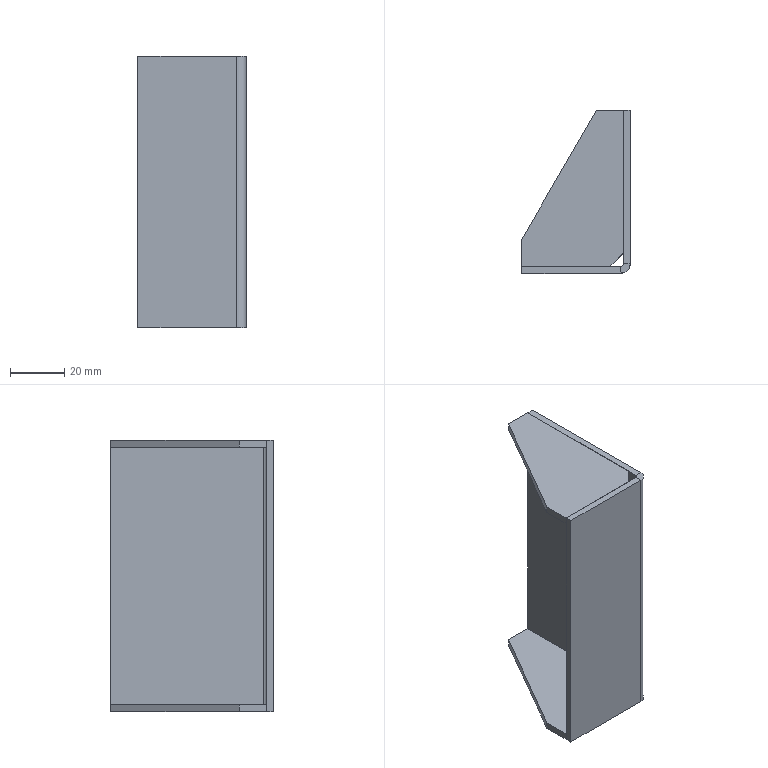Part | SolidWorks | features BaseBody 3 | 3 solids | 30 faces | box 40 x 60 x 100 mm | volume 31587 mm3 | plane 28 | cylinder 2 | commonest cylinder face diameters 2 x1 7 x1
STEP:
#1=CARTESIAN_POINT('',(-3.5,-57.5,-50.));
#2=VERTEX_POINT('',#1);
#3=CARTESIAN_POINT('',(-40.,-57.5,-50.));
#4=VERTEX_POINT('',#3);
#5=CARTESIAN_POINT('',(0.,-57.5,-50.));
#6=DIRECTION('',(-1.,0.,0.));
#7=VECTOR('',#6,1000.);
#8=LINE('',#5,#7);
#9=EDGE_CURVE('',#2,#4,#8,.T.);
#10=ORIENTED_EDGE('',*,*,#9,.F.);
#11=CARTESIAN_POINT('',(-3.5,-60.,-50.));
#12=VERTEX_POINT('',#11);
#13=CARTESIAN_POINT('',(-3.5,-57.5,-50.));
#14=DIRECTION('',(0.,-1.,0.));
#15=VECTOR('',#14,1000.);
#16=LINE('',#13,#15);
#17=EDGE_CURVE('',#2,#12,#16,.T.);
#18=ORIENTED_EDGE('',*,*,#17,.T.);
#19=CARTESIAN_POINT('',(-40.,-60.,-50.));
#20=VERTEX_POINT('',#19);
#21=CARTESIAN_POINT('',(0.,-60.,-50.));
#22=DIRECTION('',(-1.,0.,0.));
#23=VECTOR('',#22,1000.);
#24=LINE('',#21,#23);
#25=EDGE_CURVE('',#12,#20,#24,.T.);
#26=ORIENTED_EDGE('',*,*,#25,.T.);
#27=CARTESIAN_POINT('',(-40.,-60.,-50.));
#28=DIRECTION('',(0.,1.,0.));
#29=VECTOR('',#28,1000.);
#30=LINE('',#27,#29);
#31=EDGE_CURVE('',#20,#4,#30,.T.);
#32=ORIENTED_EDGE('',*,*,#31,.T.);
#33=EDGE_LOOP('',(#10,#18,#26,#32));
#34=FACE_OUTER_BOUND('',#33,.T.);
#35=CARTESIAN_POINT('',(-3.5,-56.5,-50.));
#36=DIRECTION('',(0.,0.,1.));
#37=DIRECTION('',(1.,0.,0.));
#38=AXIS2_PLACEMENT_3D('',#35,#36,#37);
#39=PLANE('',#38);
#40=ADVANCED_FACE('',(#34),#39,.F.);
#41=CARTESIAN_POINT('',(-2.5,0.,50.));
#42=VERTEX_POINT('',#41);
#43=CARTESIAN_POINT('',(-2.5,-56.5,50.));
#44=VERTEX_POINT('',#43);
#45=CARTESIAN_POINT('',(-2.5,0.,50.));
#46=DIRECTION('',(0.,-1.,0.));
#47=VECTOR('',#46,1000.);
#48=LINE('',#45,#47);
#49=EDGE_CURVE('',#42,#44,#48,.T.);
#50=ORIENTED_EDGE('',*,*,#49,.T.);
#51=CARTESIAN_POINT('',(0.,-56.5,50.));
#52=VERTEX_POINT('',#51);
#53=CARTESIAN_POINT('',(-2.5,-56.5,50.));
#54=DIRECTION('',(1.,0.,0.));
#55=VECTOR('',#54,1000.);
#56=LINE('',#53,#55);
#57=EDGE_CURVE('',#44,#52,#56,.T.);
#58=ORIENTED_EDGE('',*,*,#57,.T.);
#59=CARTESIAN_POINT('',(0.,0.,50.));
#60=VERTEX_POINT('',#59);
#61=CARTESIAN_POINT('',(0.,0.,50.));
#62=DIRECTION('',(0.,-1.,0.));
#63=VECTOR('',#62,1000.);
#64=LINE('',#61,#63);
#65=EDGE_CURVE('',#60,#52,#64,.T.);
#66=ORIENTED_EDGE('',*,*,#65,.F.);
#67=CARTESIAN_POINT('',(-2.5,0.,50.));
#68=DIRECTION('',(1.,0.,0.));
#69=VECTOR('',#68,1000.);
#70=LINE('',#67,#69);
#71=EDGE_CURVE('',#42,#60,#70,.T.);
#72=ORIENTED_EDGE('',*,*,#71,.F.);
#73=EDGE_LOOP('',(#50,#58,#66,#72));
#74=FACE_OUTER_BOUND('',#73,.T.);
#75=CARTESIAN_POINT('',(-3.5,-56.5,50.));
#76=DIRECTION('',(0.,0.,1.));
#77=DIRECTION('',(1.,0.,0.));
#78=AXIS2_PLACEMENT_3D('',#75,#76,#77);
#79=PLANE('',#78);
#80=ADVANCED_FACE('',(#74),#79,.T.);
#81=CARTESIAN_POINT('',(-2.5,-56.5,-50.));
#82=VERTEX_POINT('',#81);
#83=CARTESIAN_POINT('',(-3.5,-56.5,-50.));
#84=DIRECTION('',(0.,0.,-1.));
#85=DIRECTION('',(1.,0.,0.));
#86=AXIS2_PLACEMENT_3D('',#83,#84,#85);
#87=CIRCLE('',#86,1.);
#88=EDGE_CURVE('',#82,#2,#87,.T.);
#89=ORIENTED_EDGE('',*,*,#88,.T.);
#90=CARTESIAN_POINT('',(-3.5,-57.5,50.));
#91=VERTEX_POINT('',#90);
#92=CARTESIAN_POINT('',(-3.5,-57.5,50.));
#93=DIRECTION('',(0.,0.,-1.));
#94=VECTOR('',#93,1000.);
#95=LINE('',#92,#94);
#96=EDGE_CURVE('',#91,#2,#95,.T.);
#97=ORIENTED_EDGE('',*,*,#96,.F.);
#98=CARTESIAN_POINT('',(-3.5,-56.5,50.));
#99=DIRECTION('',(0.,0.,-1.));
#100=DIRECTION('',(1.,0.,0.));
#101=AXIS2_PLACEMENT_3D('',#98,#99,#100);
#102=CIRCLE('',#101,1.);
#103=EDGE_CURVE('',#44,#91,#102,.T.);
#104=ORIENTED_EDGE('',*,*,#103,.F.);
#105=CARTESIAN_POINT('',(-2.5,-56.5,50.));
#106=DIRECTION('',(0.,0.,-1.));
#107=VECTOR('',#106,1000.);
#108=LINE('',#105,#107);
#109=EDGE_CURVE('',#44,#82,#108,.T.);
#110=ORIENTED_EDGE('',*,*,#109,.T.);
#111=EDGE_LOOP('',(#89,#97,#104,#110));
#112=FACE_OUTER_BOUND('',#111,.T.);
#113=CARTESIAN_POINT('',(-3.5,-56.5,50.));
#114=DIRECTION('',(0.,0.,-1.));
#115=DIRECTION('',(-1.,0.,0.));
#116=AXIS2_PLACEMENT_3D('',#113,#114,#115);
#117=CYLINDRICAL_SURFACE('',#116,1.);
#118=ADVANCED_FACE('',(#112),#117,.F.);
#119=CARTESIAN_POINT('',(-2.5,0.,-50.));
#120=VERTEX_POINT('',#119);
#121=CARTESIAN_POINT('',(-2.5,0.,-50.));
#122=DIRECTION('',(0.,-1.,0.));
#123=VECTOR('',#122,1000.);
#124=LINE('',#121,#123);
#125=EDGE_CURVE('',#120,#82,#124,.T.);
#126=ORIENTED_EDGE('',*,*,#125,.T.);
#127=ORIENTED_EDGE('',*,*,#109,.F.);
#128=ORIENTED_EDGE('',*,*,#49,.F.);
#129=CARTESIAN_POINT('',(-2.5,0.,50.));
#130=DIRECTION('',(0.,0.,-1.));
#131=VECTOR('',#130,1000.);
#132=LINE('',#129,#131);
#133=EDGE_CURVE('',#42,#120,#132,.T.);
#134=ORIENTED_EDGE('',*,*,#133,.T.);
#135=EDGE_LOOP('',(#126,#127,#128,#134));
#136=FACE_OUTER_BOUND('',#135,.T.);
#137=CARTESIAN_POINT('',(-2.5,0.,50.));
#138=DIRECTION('',(1.,0.,0.));
#139=DIRECTION('',(0.,1.,0.));
#140=AXIS2_PLACEMENT_3D('',#137,#138,#139);
#141=PLANE('',#140);
#142=ADVANCED_FACE('',(#136),#141,.F.);
#143=CARTESIAN_POINT('',(0.,0.,-50.));
#144=VERTEX_POINT('',#143);
#145=CARTESIAN_POINT('',(-2.5,0.,-50.));
#146=DIRECTION('',(1.,0.,0.));
#147=VECTOR('',#146,1000.);
#148=LINE('',#145,#147);
#149=EDGE_CURVE('',#120,#144,#148,.T.);
#150=ORIENTED_EDGE('',*,*,#149,.F.);
#151=ORIENTED_EDGE('',*,*,#133,.F.);
#152=ORIENTED_EDGE('',*,*,#71,.T.);
#153=CARTESIAN_POINT('',(0.,0.,50.));
#154=DIRECTION('',(0.,0.,-1.));
#155=VECTOR('',#154,1000.);
#156=LINE('',#153,#155);
#157=EDGE_CURVE('',#60,#144,#156,.T.);
#158=ORIENTED_EDGE('',*,*,#157,.T.);
#159=EDGE_LOOP('',(#150,#151,#152,#158));
#160=FACE_OUTER_BOUND('',#159,.T.);
#161=CARTESIAN_POINT('',(-2.5,0.,50.));
#162=DIRECTION('',(0.,1.,0.));
#163=DIRECTION('',(1.,0.,0.));
#164=AXIS2_PLACEMENT_3D('',#161,#162,#163);
#165=PLANE('',#164);
#166=ADVANCED_FACE('',(#160),#165,.T.);
#167=CARTESIAN_POINT('',(0.,-56.5,-50.));
#168=VERTEX_POINT('',#167);
#169=CARTESIAN_POINT('',(0.,0.,-50.));
#170=DIRECTION('',(0.,-1.,0.));
#171=VECTOR('',#170,1000.);
#172=LINE('',#169,#171);
#173=EDGE_CURVE('',#144,#168,#172,.T.);
#174=ORIENTED_EDGE('',*,*,#173,.F.);
#175=ORIENTED_EDGE('',*,*,#157,.F.);
#176=ORIENTED_EDGE('',*,*,#65,.T.);
#177=CARTESIAN_POINT('',(0.,-56.5,50.));
#178=DIRECTION('',(0.,0.,-1.));
#179=VECTOR('',#178,1000.);
#180=LINE('',#177,#179);
#181=EDGE_CURVE('',#52,#168,#180,.T.);
#182=ORIENTED_EDGE('',*,*,#181,.T.);
#183=EDGE_LOOP('',(#174,#175,#176,#182));
#184=FACE_OUTER_BOUND('',#183,.T.);
#185=CARTESIAN_POINT('',(0.,0.,50.));
#186=DIRECTION('',(1.,0.,0.));
#187=DIRECTION('',(0.,1.,0.));
#188=AXIS2_PLACEMENT_3D('',#185,#186,#187);
#189=PLANE('',#188);
#190=ADVANCED_FACE('',(#184),#189,.T.);
#191=CARTESIAN_POINT('',(-3.5,-56.5,-50.));
#192=DIRECTION('',(0.,0.,-1.));
#193=DIRECTION('',(1.,0.,0.));
#194=AXIS2_PLACEMENT_3D('',#191,#192,#193);
#195=CIRCLE('',#194,3.5);
#196=EDGE_CURVE('',#168,#12,#195,.T.);
#197=ORIENTED_EDGE('',*,*,#196,.F.);
#198=ORIENTED_EDGE('',*,*,#181,.F.);
#199=CARTESIAN_POINT('',(-3.5,-60.,50.));
#200=VERTEX_POINT('',#199);
#201=CARTESIAN_POINT('',(-3.5,-56.5,50.));
#202=DIRECTION('',(0.,0.,-1.));
#203=DIRECTION('',(1.,0.,0.));
#204=AXIS2_PLACEMENT_3D('',#201,#202,#203);
#205=CIRCLE('',#204,3.5);
#206=EDGE_CURVE('',#52,#200,#205,.T.);
#207=ORIENTED_EDGE('',*,*,#206,.T.);
#208=CARTESIAN_POINT('',(-3.5,-60.,50.));
#209=DIRECTION('',(0.,0.,-1.));
#210=VECTOR('',#209,1000.);
#211=LINE('',#208,#210);
#212=EDGE_CURVE('',#200,#12,#211,.T.);
#213=ORIENTED_EDGE('',*,*,#212,.T.);
#214=EDGE_LOOP('',(#197,#198,#207,#213));
#215=FACE_OUTER_BOUND('',#214,.T.);
#216=CARTESIAN_POINT('',(-3.5,-56.5,50.));
#217=DIRECTION('',(0.,0.,-1.));
#218=DIRECTION('',(-1.,0.,0.));
#219=AXIS2_PLACEMENT_3D('',#216,#217,#218);
#220=CYLINDRICAL_SURFACE('',#219,3.5);
#221=ADVANCED_FACE('',(#215),#220,.T.);
#222=ORIENTED_EDGE('',*,*,#25,.F.);
#223=ORIENTED_EDGE('',*,*,#212,.F.);
#224=CARTESIAN_POINT('',(-40.,-60.,50.));
#225=VERTEX_POINT('',#224);
#226=CARTESIAN_POINT('',(0.,-60.,50.));
#227=DIRECTION('',(-1.,0.,0.));
#228=VECTOR('',#227,1000.);
#229=LINE('',#226,#228);
#230=EDGE_CURVE('',#200,#225,#229,.T.);
#231=ORIENTED_EDGE('',*,*,#230,.T.);
#232=CARTESIAN_POINT('',(-40.,-60.,50.));
#233=DIRECTION('',(0.,0.,-1.));
#234=VECTOR('',#233,1000.);
#235=LINE('',#232,#234);
#236=EDGE_CURVE('',#225,#20,#235,.T.);
#237=ORIENTED_EDGE('',*,*,#236,.T.);
#238=EDGE_LOOP('',(#222,#223,#231,#237));
#239=FACE_OUTER_BOUND('',#238,.T.);
#240=CARTESIAN_POINT('',(0.,-60.,50.));
#241=DIRECTION('',(0.,-1.,0.));
#242=DIRECTION('',(0.,0.,-1.));
#243=AXIS2_PLACEMENT_3D('',#240,#241,#242);
#244=PLANE('',#243);
#245=ADVANCED_FACE('',(#239),#244,.T.);
#246=ORIENTED_EDGE('',*,*,#31,.F.);
#247=ORIENTED_EDGE('',*,*,#236,.F.);
#248=CARTESIAN_POINT('',(-40.,-57.5,50.));
#249=VERTEX_POINT('',#248);
#250=CARTESIAN_POINT('',(-40.,-60.,50.));
#251=DIRECTION('',(0.,1.,0.));
#252=VECTOR('',#251,1000.);
#253=LINE('',#250,#252);
#254=EDGE_CURVE('',#225,#249,#253,.T.);
#255=ORIENTED_EDGE('',*,*,#254,.T.);
#256=CARTESIAN_POINT('',(-40.,-57.5,50.));
#257=DIRECTION('',(0.,0.,-1.));
#258=VECTOR('',#257,1000.);
#259=LINE('',#256,#258);
#260=EDGE_CURVE('',#249,#4,#259,.T.);
#261=ORIENTED_EDGE('',*,*,#260,.T.);
#262=EDGE_LOOP('',(#246,#247,#255,#261));
#263=FACE_OUTER_BOUND('',#262,.T.);
#264=CARTESIAN_POINT('',(-40.,-60.,50.));
#265=DIRECTION('',(-1.,0.,0.));
#266=DIRECTION('',(0.,0.,1.));
#267=AXIS2_PLACEMENT_3D('',#264,#265,#266);
#268=PLANE('',#267);
#269=ADVANCED_FACE('',(#263),#268,.T.);
#270=ORIENTED_EDGE('',*,*,#9,.T.);
#271=ORIENTED_EDGE('',*,*,#260,.F.);
#272=CARTESIAN_POINT('',(0.,-57.5,50.));
#273=DIRECTION('',(-1.,0.,0.));
#274=VECTOR('',#273,1000.);
#275=LINE('',#272,#274);
#276=EDGE_CURVE('',#91,#249,#275,.T.);
#277=ORIENTED_EDGE('',*,*,#276,.F.);
#278=ORIENTED_EDGE('',*,*,#96,.T.);
#279=EDGE_LOOP('',(#270,#271,#277,#278));
#280=FACE_OUTER_BOUND('',#279,.T.);
#281=CARTESIAN_POINT('',(0.,-57.5,50.));
#282=DIRECTION('',(0.,-1.,0.));
#283=DIRECTION('',(0.,0.,-1.));
#284=AXIS2_PLACEMENT_3D('',#281,#282,#283);
#285=PLANE('',#284);
#286=ADVANCED_FACE('',(#280),#285,.F.);
#287=ORIENTED_EDGE('',*,*,#173,.T.);
#288=CARTESIAN_POINT('',(0.,-56.5,-50.));
#289=DIRECTION('',(-1.,0.,0.));
#290=VECTOR('',#289,1000.);
#291=LINE('',#288,#290);
#292=EDGE_CURVE('',#168,#82,#291,.T.);
#293=ORIENTED_EDGE('',*,*,#292,.T.);
#294=ORIENTED_EDGE('',*,*,#125,.F.);
#295=ORIENTED_EDGE('',*,*,#149,.T.);
#296=EDGE_LOOP('',(#287,#293,#294,#295));
#297=FACE_OUTER_BOUND('',#296,.T.);
#298=CARTESIAN_POINT('',(-3.5,-57.5,-50.));
#299=DIRECTION('',(0.,0.,-1.));
#300=DIRECTION('',(0.,-1.,0.));
#301=AXIS2_PLACEMENT_3D('',#298,#299,#300);
#302=PLANE('',#301);
#303=ADVANCED_FACE('',(#297),#302,.T.);
#304=ORIENTED_EDGE('',*,*,#292,.F.);
#305=ORIENTED_EDGE('',*,*,#196,.T.);
#306=ORIENTED_EDGE('',*,*,#17,.F.);
#307=ORIENTED_EDGE('',*,*,#88,.F.);
#308=EDGE_LOOP('',(#304,#305,#306,#307));
#309=FACE_OUTER_BOUND('',#308,.T.);
#310=CARTESIAN_POINT('',(0.,-56.5,-50.));
#311=DIRECTION('',(0.,0.,-1.));
#312=DIRECTION('',(0.,-1.,0.));
#313=AXIS2_PLACEMENT_3D('',#310,#311,#312);
#314=PLANE('',#313);
#315=ADVANCED_FACE('',(#309),#314,.T.);
#316=ORIENTED_EDGE('',*,*,#230,.F.);
#317=CARTESIAN_POINT('',(-3.5,-60.,50.));
#318=DIRECTION('',(0.,1.,0.));
#319=VECTOR('',#318,1000.);
#320=LINE('',#317,#319);
#321=EDGE_CURVE('',#200,#91,#320,.T.);
#322=ORIENTED_EDGE('',*,*,#321,.T.);
#323=ORIENTED_EDGE('',*,*,#276,.T.);
#324=ORIENTED_EDGE('',*,*,#254,.F.);
#325=EDGE_LOOP('',(#316,#322,#323,#324));
#326=FACE_OUTER_BOUND('',#325,.T.);
#327=CARTESIAN_POINT('',(-2.5,-56.5,50.));
#328=DIRECTION('',(0.,0.,1.));
#329=DIRECTION('',(1.,0.,0.));
#330=AXIS2_PLACEMENT_3D('',#327,#328,#329);
#331=PLANE('',#330);
#332=ADVANCED_FACE('',(#326),#331,.T.);
#333=ORIENTED_EDGE('',*,*,#321,.F.);
#334=ORIENTED_EDGE('',*,*,#206,.F.);
#335=ORIENTED_EDGE('',*,*,#57,.F.);
#336=ORIENTED_EDGE('',*,*,#103,.T.);
#337=EDGE_LOOP('',(#333,#334,#335,#336));
#338=FACE_OUTER_BOUND('',#337,.T.);
#339=CARTESIAN_POINT('',(-3.5,-60.,50.));
#340=DIRECTION('',(0.,0.,1.));
#341=DIRECTION('',(1.,0.,0.));
#342=AXIS2_PLACEMENT_3D('',#339,#340,#341);
#343=PLANE('',#342);
#344=ADVANCED_FACE('',(#338),#343,.T.);
#345=CLOSED_SHELL('',(#40,#80,#118,#142,#166,#190,#221,#245,#269,#286,#303,#315,#332,#344));
#346=MANIFOLD_SOLID_BREP('',#345);
#347=CARTESIAN_POINT('',(-2.5,0.,-50.));
#348=VERTEX_POINT('',#347);
#349=CARTESIAN_POINT('',(-2.5,-52.5,-50.));
#350=VERTEX_POINT('',#349);
#351=CARTESIAN_POINT('',(-2.5,-52.5,-50.));
#352=DIRECTION('',(0.,-1.,0.));
#353=VECTOR('',#352,1000.);
#354=LINE('',#351,#353);
#355=EDGE_CURVE('',#348,#350,#354,.T.);
#356=ORIENTED_EDGE('',*,*,#355,.T.);
#357=CARTESIAN_POINT('',(-7.5,-57.5,-50.));
#358=VERTEX_POINT('',#357);
#359=CARTESIAN_POINT('',(-7.5,-57.5,-50.));
#360=DIRECTION('',(-0.7071,-0.7071,0.));
#361=VECTOR('',#360,1000.);
#362=LINE('',#359,#361);
#363=EDGE_CURVE('',#350,#358,#362,.T.);
#364=ORIENTED_EDGE('',*,*,#363,.T.);
#365=CARTESIAN_POINT('',(-40.,-57.5,-50.));
#366=VERTEX_POINT('',#365);
#367=CARTESIAN_POINT('',(-40.,-57.5,-50.));
#368=DIRECTION('',(-1.,0.,0.));
#369=VECTOR('',#368,1000.);
#370=LINE('',#367,#369);
#371=EDGE_CURVE('',#358,#366,#370,.T.);
#372=ORIENTED_EDGE('',*,*,#371,.T.);
#373=CARTESIAN_POINT('',(-40.,-47.5,-50.));
#374=VERTEX_POINT('',#373);
#375=CARTESIAN_POINT('',(-40.,-47.5,-50.));
#376=DIRECTION('',(0.,1.,0.));
#377=VECTOR('',#376,1000.);
#378=LINE('',#375,#377);
#379=EDGE_CURVE('',#366,#374,#378,.T.);
#380=ORIENTED_EDGE('',*,*,#379,.T.);
#381=CARTESIAN_POINT('',(-12.5,0.,-50.));
#382=VERTEX_POINT('',#381);
#383=CARTESIAN_POINT('',(-12.5,0.,-50.));
#384=DIRECTION('',(0.501,0.8654,0.));
#385=VECTOR('',#384,1000.);
#386=LINE('',#383,#385);
#387=EDGE_CURVE('',#374,#382,#386,.T.);
#388=ORIENTED_EDGE('',*,*,#387,.T.);
#389=CARTESIAN_POINT('',(-2.5,0.,-50.));
#390=DIRECTION('',(1.,0.,0.));
#391=VECTOR('',#390,1000.);
#392=LINE('',#389,#391);
#393=EDGE_CURVE('',#382,#348,#392,.T.);
#394=ORIENTED_EDGE('',*,*,#393,.T.);
#395=EDGE_LOOP('',(#356,#364,#372,#380,#388,#394));
#396=FACE_OUTER_BOUND('',#395,.T.);
#397=CARTESIAN_POINT('',(0.,0.,-50.));
#398=DIRECTION('',(0.,0.,1.));
#399=DIRECTION('',(1.,0.,0.));
#400=AXIS2_PLACEMENT_3D('',#397,#398,#399);
#401=PLANE('',#400);
#402=ADVANCED_FACE('',(#396),#401,.F.);
#403=CARTESIAN_POINT('',(-2.5,0.,-47.5));
#404=VERTEX_POINT('',#403);
#405=CARTESIAN_POINT('',(-2.5,-52.5,-47.5));
#406=VERTEX_POINT('',#405);
#407=CARTESIAN_POINT('',(-2.5,-52.5,-47.5));
#408=DIRECTION('',(0.,-1.,0.));
#409=VECTOR('',#408,1000.);
#410=LINE('',#407,#409);
#411=EDGE_CURVE('',#404,#406,#410,.T.);
#412=ORIENTED_EDGE('',*,*,#411,.F.);
#413=CARTESIAN_POINT('',(-12.5,0.,-47.5));
#414=VERTEX_POINT('',#413);
#415=CARTESIAN_POINT('',(-2.5,0.,-47.5));
#416=DIRECTION('',(1.,0.,0.));
#417=VECTOR('',#416,1000.);
#418=LINE('',#415,#417);
#419=EDGE_CURVE('',#414,#404,#418,.T.);
#420=ORIENTED_EDGE('',*,*,#419,.F.);
#421=CARTESIAN_POINT('',(-40.,-47.5,-47.5));
#422=VERTEX_POINT('',#421);
#423=CARTESIAN_POINT('',(-12.5,0.,-47.5));
#424=DIRECTION('',(0.501,0.8654,0.));
#425=VECTOR('',#424,1000.);
#426=LINE('',#423,#425);
#427=EDGE_CURVE('',#422,#414,#426,.T.);
#428=ORIENTED_EDGE('',*,*,#427,.F.);
#429=CARTESIAN_POINT('',(-40.,-57.5,-47.5));
#430=VERTEX_POINT('',#429);
#431=CARTESIAN_POINT('',(-40.,-47.5,-47.5));
#432=DIRECTION('',(0.,1.,0.));
#433=VECTOR('',#432,1000.);
#434=LINE('',#431,#433);
#435=EDGE_CURVE('',#430,#422,#434,.T.);
#436=ORIENTED_EDGE('',*,*,#435,.F.);
#437=CARTESIAN_POINT('',(-7.5,-57.5,-47.5));
#438=VERTEX_POINT('',#437);
#439=CARTESIAN_POINT('',(-40.,-57.5,-47.5));
#440=DIRECTION('',(-1.,0.,0.));
#441=VECTOR('',#440,1000.);
#442=LINE('',#439,#441);
#443=EDGE_CURVE('',#438,#430,#442,.T.);
#444=ORIENTED_EDGE('',*,*,#443,.F.);
#445=CARTESIAN_POINT('',(-7.5,-57.5,-47.5));
#446=DIRECTION('',(-0.7071,-0.7071,0.));
#447=VECTOR('',#446,1000.);
#448=LINE('',#445,#447);
#449=EDGE_CURVE('',#406,#438,#448,.T.);
#450=ORIENTED_EDGE('',*,*,#449,.F.);
#451=EDGE_LOOP('',(#412,#420,#428,#436,#444,#450));
#452=FACE_OUTER_BOUND('',#451,.T.);
#453=CARTESIAN_POINT('',(0.,0.,-47.5));
#454=DIRECTION('',(0.,0.,1.));
#455=DIRECTION('',(1.,0.,0.));
#456=AXIS2_PLACEMENT_3D('',#453,#454,#455);
#457=PLANE('',#456);
#458=ADVANCED_FACE('',(#452),#457,.T.);
#459=ORIENTED_EDGE('',*,*,#363,.F.);
#460=CARTESIAN_POINT('',(-2.5,-52.5,-47.5));
#461=DIRECTION('',(0.,0.,-1.));
#462=VECTOR('',#461,1000.);
#463=LINE('',#460,#462);
#464=EDGE_CURVE('',#406,#350,#463,.T.);
#465=ORIENTED_EDGE('',*,*,#464,.F.);
#466=ORIENTED_EDGE('',*,*,#449,.T.);
#467=CARTESIAN_POINT('',(-7.5,-57.5,-47.5));
#468=DIRECTION('',(0.,0.,-1.));
#469=VECTOR('',#468,1000.);
#470=LINE('',#467,#469);
#471=EDGE_CURVE('',#438,#358,#470,.T.);
#472=ORIENTED_EDGE('',*,*,#471,.T.);
#473=EDGE_LOOP('',(#459,#465,#466,#472));
#474=FACE_OUTER_BOUND('',#473,.T.);
#475=CARTESIAN_POINT('',(-7.5,-57.5,-47.5));
#476=DIRECTION('',(0.7071,-0.7071,0.));
#477=DIRECTION('',(0.,0.,-1.));
#478=AXIS2_PLACEMENT_3D('',#475,#476,#477);
#479=PLANE('',#478);
#480=ADVANCED_FACE('',(#474),#479,.T.);
#481=ORIENTED_EDGE('',*,*,#371,.F.);
#482=ORIENTED_EDGE('',*,*,#471,.F.);
#483=ORIENTED_EDGE('',*,*,#443,.T.);
#484=CARTESIAN_POINT('',(-40.,-57.5,-47.5));
#485=DIRECTION('',(0.,0.,-1.));
#486=VECTOR('',#485,1000.);
#487=LINE('',#484,#486);
#488=EDGE_CURVE('',#430,#366,#487,.T.);
#489=ORIENTED_EDGE('',*,*,#488,.T.);
#490=EDGE_LOOP('',(#481,#482,#483,#489));
#491=FACE_OUTER_BOUND('',#490,.T.);
#492=CARTESIAN_POINT('',(-40.,-57.5,-47.5));
#493=DIRECTION('',(0.,-1.,0.));
#494=DIRECTION('',(0.,0.,-1.));
#495=AXIS2_PLACEMENT_3D('',#492,#493,#494);
#496=PLANE('',#495);
#497=ADVANCED_FACE('',(#491),#496,.T.);
#498=ORIENTED_EDGE('',*,*,#379,.F.);
#499=ORIENTED_EDGE('',*,*,#488,.F.);
#500=ORIENTED_EDGE('',*,*,#435,.T.);
#501=CARTESIAN_POINT('',(-40.,-47.5,-47.5));
#502=DIRECTION('',(0.,0.,-1.));
#503=VECTOR('',#502,1000.);
#504=LINE('',#501,#503);
#505=EDGE_CURVE('',#422,#374,#504,.T.);
#506=ORIENTED_EDGE('',*,*,#505,.T.);
#507=EDGE_LOOP('',(#498,#499,#500,#506));
#508=FACE_OUTER_BOUND('',#507,.T.);
#509=CARTESIAN_POINT('',(-40.,-47.5,-47.5));
#510=DIRECTION('',(-1.,0.,0.));
#511=DIRECTION('',(0.,0.,1.));
#512=AXIS2_PLACEMENT_3D('',#509,#510,#511);
#513=PLANE('',#512);
#514=ADVANCED_FACE('',(#508),#513,.T.);
#515=ORIENTED_EDGE('',*,*,#387,.F.);
#516=ORIENTED_EDGE('',*,*,#505,.F.);
#517=ORIENTED_EDGE('',*,*,#427,.T.);
#518=CARTESIAN_POINT('',(-12.5,0.,-47.5));
#519=DIRECTION('',(0.,0.,-1.));
#520=VECTOR('',#519,1000.);
#521=LINE('',#518,#520);
#522=EDGE_CURVE('',#414,#382,#521,.T.);
#523=ORIENTED_EDGE('',*,*,#522,.T.);
#524=EDGE_LOOP('',(#515,#516,#517,#523));
#525=FACE_OUTER_BOUND('',#524,.T.);
#526=CARTESIAN_POINT('',(-12.5,0.,-47.5));
#527=DIRECTION('',(-0.8654,0.501,0.));
#528=DIRECTION('',(0.,0.,1.));
#529=AXIS2_PLACEMENT_3D('',#526,#527,#528);
#530=PLANE('',#529);
#531=ADVANCED_FACE('',(#525),#530,.T.);
#532=ORIENTED_EDGE('',*,*,#393,.F.);
#533=ORIENTED_EDGE('',*,*,#522,.F.);
#534=ORIENTED_EDGE('',*,*,#419,.T.);
#535=CARTESIAN_POINT('',(-2.5,0.,-47.5));
#536=DIRECTION('',(0.,0.,-1.));
#537=VECTOR('',#536,1000.);
#538=LINE('',#535,#537);
#539=EDGE_CURVE('',#404,#348,#538,.T.);
#540=ORIENTED_EDGE('',*,*,#539,.T.);
#541=EDGE_LOOP('',(#532,#533,#534,#540));
#542=FACE_OUTER_BOUND('',#541,.T.);
#543=CARTESIAN_POINT('',(-2.5,0.,-47.5));
#544=DIRECTION('',(0.,1.,0.));
#545=DIRECTION('',(1.,0.,0.));
#546=AXIS2_PLACEMENT_3D('',#543,#544,#545);
#547=PLANE('',#546);
#548=ADVANCED_FACE('',(#542),#547,.T.);
#549=ORIENTED_EDGE('',*,*,#355,.F.);
#550=ORIENTED_EDGE('',*,*,#539,.F.);
#551=ORIENTED_EDGE('',*,*,#411,.T.);
#552=ORIENTED_EDGE('',*,*,#464,.T.);
#553=EDGE_LOOP('',(#549,#550,#551,#552));
#554=FACE_OUTER_BOUND('',#553,.T.);
#555=CARTESIAN_POINT('',(-2.5,-52.5,-47.5));
#556=DIRECTION('',(1.,0.,0.));
#557=DIRECTION('',(0.,1.,0.));
#558=AXIS2_PLACEMENT_3D('',#555,#556,#557);
#559=PLANE('',#558);
#560=ADVANCED_FACE('',(#554),#559,.T.);
#561=CLOSED_SHELL('',(#402,#458,#480,#497,#514,#531,#548,#560));
#562=MANIFOLD_SOLID_BREP('',#561);
#563=CARTESIAN_POINT('',(-2.5,0.,50.));
#564=VERTEX_POINT('',#563);
#565=CARTESIAN_POINT('',(-2.5,-52.5,50.));
#566=VERTEX_POINT('',#565);
#567=CARTESIAN_POINT('',(-2.5,-52.5,50.));
#568=DIRECTION('',(0.,-1.,0.));
#569=VECTOR('',#568,1000.);
#570=LINE('',#567,#569);
#571=EDGE_CURVE('',#564,#566,#570,.T.);
#572=ORIENTED_EDGE('',*,*,#571,.F.);
#573=CARTESIAN_POINT('',(-12.5,0.,50.));
#574=VERTEX_POINT('',#573);
#575=CARTESIAN_POINT('',(-2.5,0.,50.));
#576=DIRECTION('',(1.,0.,0.));
#577=VECTOR('',#576,1000.);
#578=LINE('',#575,#577);
#579=EDGE_CURVE('',#574,#564,#578,.T.);
#580=ORIENTED_EDGE('',*,*,#579,.F.);
#581=CARTESIAN_POINT('',(-40.,-47.5,50.));
#582=VERTEX_POINT('',#581);
#583=CARTESIAN_POINT('',(-12.5,0.,50.));
#584=DIRECTION('',(0.501,0.8654,0.));
#585=VECTOR('',#584,1000.);
#586=LINE('',#583,#585);
#587=EDGE_CURVE('',#582,#574,#586,.T.);
#588=ORIENTED_EDGE('',*,*,#587,.F.);
#589=CARTESIAN_POINT('',(-40.,-57.5,50.));
#590=VERTEX_POINT('',#589);
#591=CARTESIAN_POINT('',(-40.,-47.5,50.));
#592=DIRECTION('',(0.,1.,0.));
#593=VECTOR('',#592,1000.);
#594=LINE('',#591,#593);
#595=EDGE_CURVE('',#590,#582,#594,.T.);
#596=ORIENTED_EDGE('',*,*,#595,.F.);
#597=CARTESIAN_POINT('',(-7.5,-57.5,50.));
#598=VERTEX_POINT('',#597);
#599=CARTESIAN_POINT('',(-40.,-57.5,50.));
#600=DIRECTION('',(-1.,0.,0.));
#601=VECTOR('',#600,1000.);
#602=LINE('',#599,#601);
#603=EDGE_CURVE('',#598,#590,#602,.T.);
#604=ORIENTED_EDGE('',*,*,#603,.F.);
#605=CARTESIAN_POINT('',(-7.5,-57.5,50.));
#606=DIRECTION('',(-0.7071,-0.7071,0.));
#607=VECTOR('',#606,1000.);
#608=LINE('',#605,#607);
#609=EDGE_CURVE('',#566,#598,#608,.T.);
#610=ORIENTED_EDGE('',*,*,#609,.F.);
#611=EDGE_LOOP('',(#572,#580,#588,#596,#604,#610));
#612=FACE_OUTER_BOUND('',#611,.T.);
#613=CARTESIAN_POINT('',(0.,0.,50.));
#614=DIRECTION('',(0.,0.,-1.));
#615=DIRECTION('',(0.,-1.,0.));
#616=AXIS2_PLACEMENT_3D('',#613,#614,#615);
#617=PLANE('',#616);
#618=ADVANCED_FACE('',(#612),#617,.F.);
#619=CARTESIAN_POINT('',(-2.5,0.,47.5));
#620=VERTEX_POINT('',#619);
#621=CARTESIAN_POINT('',(-2.5,-52.5,47.5));
#622=VERTEX_POINT('',#621);
#623=CARTESIAN_POINT('',(-2.5,-52.5,47.5));
#624=DIRECTION('',(0.,-1.,0.));
#625=VECTOR('',#624,1000.);
#626=LINE('',#623,#625);
#627=EDGE_CURVE('',#620,#622,#626,.T.);
#628=ORIENTED_EDGE('',*,*,#627,.T.);
#629=CARTESIAN_POINT('',(-7.5,-57.5,47.5));
#630=VERTEX_POINT('',#629);
#631=CARTESIAN_POINT('',(-7.5,-57.5,47.5));
#632=DIRECTION('',(-0.7071,-0.7071,0.));
#633=VECTOR('',#632,1000.);
#634=LINE('',#631,#633);
#635=EDGE_CURVE('',#622,#630,#634,.T.);
#636=ORIENTED_EDGE('',*,*,#635,.T.);
#637=CARTESIAN_POINT('',(-40.,-57.5,47.5));
#638=VERTEX_POINT('',#637);
#639=CARTESIAN_POINT('',(-40.,-57.5,47.5));
#640=DIRECTION('',(-1.,0.,0.));
#641=VECTOR('',#640,1000.);
#642=LINE('',#639,#641);
#643=EDGE_CURVE('',#630,#638,#642,.T.);
#644=ORIENTED_EDGE('',*,*,#643,.T.);
#645=CARTESIAN_POINT('',(-40.,-47.5,47.5));
#646=VERTEX_POINT('',#645);
#647=CARTESIAN_POINT('',(-40.,-47.5,47.5));
#648=DIRECTION('',(0.,1.,0.));
#649=VECTOR('',#648,1000.);
#650=LINE('',#647,#649);
#651=EDGE_CURVE('',#638,#646,#650,.T.);
#652=ORIENTED_EDGE('',*,*,#651,.T.);
#653=CARTESIAN_POINT('',(-12.5,0.,47.5));
#654=VERTEX_POINT('',#653);
#655=CARTESIAN_POINT('',(-12.5,0.,47.5));
#656=DIRECTION('',(0.501,0.8654,0.));
#657=VECTOR('',#656,1000.);
#658=LINE('',#655,#657);
#659=EDGE_CURVE('',#646,#654,#658,.T.);
#660=ORIENTED_EDGE('',*,*,#659,.T.);
#661=CARTESIAN_POINT('',(-2.5,0.,47.5));
#662=DIRECTION('',(1.,0.,0.));
#663=VECTOR('',#662,1000.);
#664=LINE('',#661,#663);
#665=EDGE_CURVE('',#654,#620,#664,.T.);
#666=ORIENTED_EDGE('',*,*,#665,.T.);
#667=EDGE_LOOP('',(#628,#636,#644,#652,#660,#666));
#668=FACE_OUTER_BOUND('',#667,.T.);
#669=CARTESIAN_POINT('',(0.,0.,47.5));
#670=DIRECTION('',(0.,0.,-1.));
#671=DIRECTION('',(0.,-1.,0.));
#672=AXIS2_PLACEMENT_3D('',#669,#670,#671);
#673=PLANE('',#672);
#674=ADVANCED_FACE('',(#668),#673,.T.);
#675=ORIENTED_EDGE('',*,*,#609,.T.);
#676=CARTESIAN_POINT('',(-7.5,-57.5,47.5));
#677=DIRECTION('',(0.,0.,1.));
#678=VECTOR('',#677,1000.);
#679=LINE('',#676,#678);
#680=EDGE_CURVE('',#630,#598,#679,.T.);
#681=ORIENTED_EDGE('',*,*,#680,.F.);
#682=ORIENTED_EDGE('',*,*,#635,.F.);
#683=CARTESIAN_POINT('',(-2.5,-52.5,47.5));
#684=DIRECTION('',(0.,0.,1.));
#685=VECTOR('',#684,1000.);
#686=LINE('',#683,#685);
#687=EDGE_CURVE('',#622,#566,#686,.T.);
#688=ORIENTED_EDGE('',*,*,#687,.T.);
#689=EDGE_LOOP('',(#675,#681,#682,#688));
#690=FACE_OUTER_BOUND('',#689,.T.);
#691=CARTESIAN_POINT('',(-7.5,-57.5,47.5));
#692=DIRECTION('',(0.7071,-0.7071,0.));
#693=DIRECTION('',(0.,0.,-1.));
#694=AXIS2_PLACEMENT_3D('',#691,#692,#693);
#695=PLANE('',#694);
#696=ADVANCED_FACE('',(#690),#695,.T.);
#697=ORIENTED_EDGE('',*,*,#603,.T.);
#698=CARTESIAN_POINT('',(-40.,-57.5,47.5));
#699=DIRECTION('',(0.,0.,1.));
#700=VECTOR('',#699,1000.);
#701=LINE('',#698,#700);
#702=EDGE_CURVE('',#638,#590,#701,.T.);
#703=ORIENTED_EDGE('',*,*,#702,.F.);
#704=ORIENTED_EDGE('',*,*,#643,.F.);
#705=ORIENTED_EDGE('',*,*,#680,.T.);
#706=EDGE_LOOP('',(#697,#703,#704,#705));
#707=FACE_OUTER_BOUND('',#706,.T.);
#708=CARTESIAN_POINT('',(-40.,-57.5,47.5));
#709=DIRECTION('',(0.,-1.,0.));
#710=DIRECTION('',(0.,0.,-1.));
#711=AXIS2_PLACEMENT_3D('',#708,#709,#710);
#712=PLANE('',#711);
#713=ADVANCED_FACE('',(#707),#712,.T.);
#714=ORIENTED_EDGE('',*,*,#595,.T.);
#715=CARTESIAN_POINT('',(-40.,-47.5,47.5));
#716=DIRECTION('',(0.,0.,1.));
#717=VECTOR('',#716,1000.);
#718=LINE('',#715,#717);
#719=EDGE_CURVE('',#646,#582,#718,.T.);
#720=ORIENTED_EDGE('',*,*,#719,.F.);
#721=ORIENTED_EDGE('',*,*,#651,.F.);
#722=ORIENTED_EDGE('',*,*,#702,.T.);
#723=EDGE_LOOP('',(#714,#720,#721,#722));
#724=FACE_OUTER_BOUND('',#723,.T.);
#725=CARTESIAN_POINT('',(-40.,-47.5,47.5));
#726=DIRECTION('',(-1.,0.,0.));
#727=DIRECTION('',(0.,0.,1.));
#728=AXIS2_PLACEMENT_3D('',#725,#726,#727);
#729=PLANE('',#728);
#730=ADVANCED_FACE('',(#724),#729,.T.);
#731=ORIENTED_EDGE('',*,*,#587,.T.);
#732=CARTESIAN_POINT('',(-12.5,0.,47.5));
#733=DIRECTION('',(0.,0.,1.));
#734=VECTOR('',#733,1000.);
#735=LINE('',#732,#734);
#736=EDGE_CURVE('',#654,#574,#735,.T.);
#737=ORIENTED_EDGE('',*,*,#736,.F.);
#738=ORIENTED_EDGE('',*,*,#659,.F.);
#739=ORIENTED_EDGE('',*,*,#719,.T.);
#740=EDGE_LOOP('',(#731,#737,#738,#739));
#741=FACE_OUTER_BOUND('',#740,.T.);
#742=CARTESIAN_POINT('',(-12.5,0.,47.5));
#743=DIRECTION('',(-0.8654,0.501,0.));
#744=DIRECTION('',(0.,0.,1.));
#745=AXIS2_PLACEMENT_3D('',#742,#743,#744);
#746=PLANE('',#745);
#747=ADVANCED_FACE('',(#741),#746,.T.);
#748=ORIENTED_EDGE('',*,*,#579,.T.);
#749=CARTESIAN_POINT('',(-2.5,0.,47.5));
#750=DIRECTION('',(0.,0.,1.));
#751=VECTOR('',#750,1000.);
#752=LINE('',#749,#751);
#753=EDGE_CURVE('',#620,#564,#752,.T.);
#754=ORIENTED_EDGE('',*,*,#753,.F.);
#755=ORIENTED_EDGE('',*,*,#665,.F.);
#756=ORIENTED_EDGE('',*,*,#736,.T.);
#757=EDGE_LOOP('',(#748,#754,#755,#756));
#758=FACE_OUTER_BOUND('',#757,.T.);
#759=CARTESIAN_POINT('',(-2.5,0.,47.5));
#760=DIRECTION('',(0.,1.,0.));
#761=DIRECTION('',(1.,0.,0.));
#762=AXIS2_PLACEMENT_3D('',#759,#760,#761);
#763=PLANE('',#762);
#764=ADVANCED_FACE('',(#758),#763,.T.);
#765=ORIENTED_EDGE('',*,*,#571,.T.);
#766=ORIENTED_EDGE('',*,*,#687,.F.);
#767=ORIENTED_EDGE('',*,*,#627,.F.);
#768=ORIENTED_EDGE('',*,*,#753,.T.);
#769=EDGE_LOOP('',(#765,#766,#767,#768));
#770=FACE_OUTER_BOUND('',#769,.T.);
#771=CARTESIAN_POINT('',(-2.5,-52.5,47.5));
#772=DIRECTION('',(1.,0.,0.));
#773=DIRECTION('',(0.,1.,0.));
#774=AXIS2_PLACEMENT_3D('',#771,#772,#773);
#775=PLANE('',#774);
#776=ADVANCED_FACE('',(#770),#775,.T.);
#777=CLOSED_SHELL('',(#618,#674,#696,#713,#730,#747,#764,#776));
#778=MANIFOLD_SOLID_BREP('',#777);
#779=CARTESIAN_POINT('',(0.,0.,0.));
#780=DIRECTION('',(0.,0.,1.));
#781=DIRECTION('',(1.,0.,0.));
#782=AXIS2_PLACEMENT_3D('',#779,#780,#781);
#783=(LENGTH_UNIT()NAMED_UNIT(*)SI_UNIT(.MILLI.,.METRE.));
#784=UNCERTAINTY_MEASURE_WITH_UNIT(LENGTH_MEASURE(0.00001),#783,'','');
#785=(NAMED_UNIT(*)PLANE_ANGLE_UNIT()SI_UNIT($,.RADIAN.));
#786=(NAMED_UNIT(*)SI_UNIT($,.STERADIAN.)SOLID_ANGLE_UNIT());
#787=(GEOMETRIC_REPRESENTATION_CONTEXT(3)GLOBAL_UNCERTAINTY_ASSIGNED_CONTEXT((#784))GLOBAL_UNIT_ASSIGNED_CONTEXT((#783,#785,#786))REPRESENTATION_CONTEXT('',''));
#788=ADVANCED_BREP_SHAPE_REPRESENTATION('',(#346,#562,#778,#782),#787);